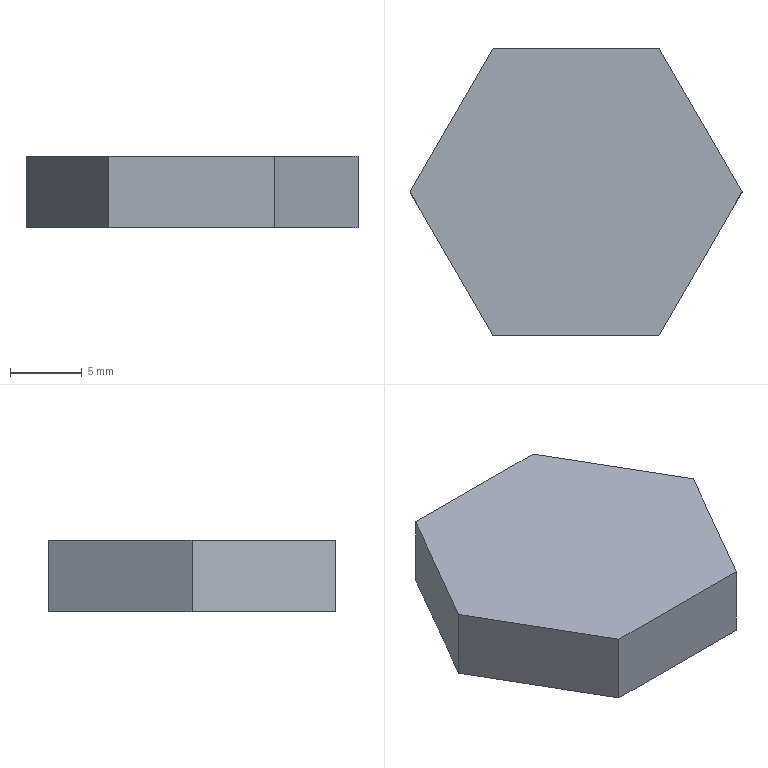Part | NX | features solid 2 | 1 solid | 8 faces | box 23.094 x 20 x 5 mm | volume 1732 mm3 | plane 8
STEP:
#1=CARTESIAN_POINT('',(20.774,205.,0.));
#2=VERTEX_POINT('',#1);
#3=CARTESIAN_POINT('',(9.226,205.,0.));
#4=VERTEX_POINT('',#3);
#5=CARTESIAN_POINT('',(-2.321,205.,0.));
#6=DIRECTION('',(-1.,0.,0.));
#7=VECTOR('',#6,1000.);
#8=LINE('',#5,#7);
#9=EDGE_CURVE('',#2,#4,#8,.T.);
#10=ORIENTED_EDGE('',*,*,#9,.F.);
#11=CARTESIAN_POINT('',(20.774,205.,-5.));
#12=VERTEX_POINT('',#11);
#13=CARTESIAN_POINT('',(20.774,205.,-5.));
#14=DIRECTION('',(0.,0.,1.));
#15=VECTOR('',#14,1000.);
#16=LINE('',#13,#15);
#17=EDGE_CURVE('',#12,#2,#16,.T.);
#18=ORIENTED_EDGE('',*,*,#17,.F.);
#19=CARTESIAN_POINT('',(9.226,205.,-5.));
#20=VERTEX_POINT('',#19);
#21=CARTESIAN_POINT('',(20.774,205.,-5.));
#22=DIRECTION('',(-1.,0.,0.));
#23=VECTOR('',#22,1000.);
#24=LINE('',#21,#23);
#25=EDGE_CURVE('',#12,#20,#24,.T.);
#26=ORIENTED_EDGE('',*,*,#25,.T.);
#27=CARTESIAN_POINT('',(9.226,205.,-5.));
#28=DIRECTION('',(0.,0.,1.));
#29=VECTOR('',#28,1000.);
#30=LINE('',#27,#29);
#31=EDGE_CURVE('',#20,#4,#30,.T.);
#32=ORIENTED_EDGE('',*,*,#31,.T.);
#33=EDGE_LOOP('',(#10,#18,#26,#32));
#34=FACE_BOUND('',#33,.T.);
#35=CARTESIAN_POINT('',(20.774,205.,-5.));
#36=DIRECTION('',(0.,1.,0.));
#37=DIRECTION('',(0.,0.,1.));
#38=AXIS2_PLACEMENT_3D('',#35,#36,#37);
#39=PLANE('',#38);
#40=ADVANCED_FACE('',(#34),#39,.T.);
#41=CARTESIAN_POINT('',(3.453,195.,0.));
#42=VERTEX_POINT('',#41);
#43=CARTESIAN_POINT('',(6.34,200.,0.));
#44=DIRECTION('',(-0.5,-0.866,0.));
#45=VECTOR('',#44,1000.);
#46=LINE('',#43,#45);
#47=EDGE_CURVE('',#4,#42,#46,.T.);
#48=ORIENTED_EDGE('',*,*,#47,.F.);
#49=ORIENTED_EDGE('',*,*,#31,.F.);
#50=CARTESIAN_POINT('',(3.453,195.,-5.));
#51=VERTEX_POINT('',#50);
#52=CARTESIAN_POINT('',(9.226,205.,-5.));
#53=DIRECTION('',(-0.5,-0.866,0.));
#54=VECTOR('',#53,1000.);
#55=LINE('',#52,#54);
#56=EDGE_CURVE('',#20,#51,#55,.T.);
#57=ORIENTED_EDGE('',*,*,#56,.T.);
#58=CARTESIAN_POINT('',(3.453,195.,-5.));
#59=DIRECTION('',(0.,0.,1.));
#60=VECTOR('',#59,1000.);
#61=LINE('',#58,#60);
#62=EDGE_CURVE('',#51,#42,#61,.T.);
#63=ORIENTED_EDGE('',*,*,#62,.T.);
#64=EDGE_LOOP('',(#48,#49,#57,#63));
#65=FACE_BOUND('',#64,.T.);
#66=CARTESIAN_POINT('',(9.226,205.,-5.));
#67=DIRECTION('',(-0.866,0.5,0.));
#68=DIRECTION('',(-0.5,-0.866,0.));
#69=AXIS2_PLACEMENT_3D('',#66,#67,#68);
#70=PLANE('',#69);
#71=ADVANCED_FACE('',(#65),#70,.T.);
#72=CARTESIAN_POINT('',(9.226,185.,0.));
#73=VERTEX_POINT('',#72);
#74=CARTESIAN_POINT('',(-2.321,205.,0.));
#75=DIRECTION('',(0.5,-0.866,0.));
#76=VECTOR('',#75,1000.);
#77=LINE('',#74,#76);
#78=EDGE_CURVE('',#42,#73,#77,.T.);
#79=ORIENTED_EDGE('',*,*,#78,.F.);
#80=ORIENTED_EDGE('',*,*,#62,.F.);
#81=CARTESIAN_POINT('',(9.226,185.,-5.));
#82=VERTEX_POINT('',#81);
#83=CARTESIAN_POINT('',(3.453,195.,-5.));
#84=DIRECTION('',(0.5,-0.866,0.));
#85=VECTOR('',#84,1000.);
#86=LINE('',#83,#85);
#87=EDGE_CURVE('',#51,#82,#86,.T.);
#88=ORIENTED_EDGE('',*,*,#87,.T.);
#89=CARTESIAN_POINT('',(9.226,185.,-5.));
#90=DIRECTION('',(0.,0.,1.));
#91=VECTOR('',#90,1000.);
#92=LINE('',#89,#91);
#93=EDGE_CURVE('',#82,#73,#92,.T.);
#94=ORIENTED_EDGE('',*,*,#93,.T.);
#95=EDGE_LOOP('',(#79,#80,#88,#94));
#96=FACE_BOUND('',#95,.T.);
#97=CARTESIAN_POINT('',(3.453,195.,-5.));
#98=DIRECTION('',(-0.866,-0.5,0.));
#99=DIRECTION('',(0.5,-0.866,0.));
#100=AXIS2_PLACEMENT_3D('',#97,#98,#99);
#101=PLANE('',#100);
#102=ADVANCED_FACE('',(#96),#101,.T.);
#103=CARTESIAN_POINT('',(20.774,185.,0.));
#104=VERTEX_POINT('',#103);
#105=CARTESIAN_POINT('',(-2.321,185.,0.));
#106=DIRECTION('',(1.,0.,0.));
#107=VECTOR('',#106,1000.);
#108=LINE('',#105,#107);
#109=EDGE_CURVE('',#73,#104,#108,.T.);
#110=ORIENTED_EDGE('',*,*,#109,.F.);
#111=ORIENTED_EDGE('',*,*,#93,.F.);
#112=CARTESIAN_POINT('',(20.774,185.,-5.));
#113=VERTEX_POINT('',#112);
#114=CARTESIAN_POINT('',(9.226,185.,-5.));
#115=DIRECTION('',(1.,0.,0.));
#116=VECTOR('',#115,1000.);
#117=LINE('',#114,#116);
#118=EDGE_CURVE('',#82,#113,#117,.T.);
#119=ORIENTED_EDGE('',*,*,#118,.T.);
#120=CARTESIAN_POINT('',(20.774,185.,-5.));
#121=DIRECTION('',(0.,0.,1.));
#122=VECTOR('',#121,1000.);
#123=LINE('',#120,#122);
#124=EDGE_CURVE('',#113,#104,#123,.T.);
#125=ORIENTED_EDGE('',*,*,#124,.T.);
#126=EDGE_LOOP('',(#110,#111,#119,#125));
#127=FACE_BOUND('',#126,.T.);
#128=CARTESIAN_POINT('',(9.226,185.,-5.));
#129=DIRECTION('',(0.,-1.,0.));
#130=DIRECTION('',(1.,0.,0.));
#131=AXIS2_PLACEMENT_3D('',#128,#129,#130);
#132=PLANE('',#131);
#133=ADVANCED_FACE('',(#127),#132,.T.);
#134=CARTESIAN_POINT('',(26.547,195.,0.));
#135=VERTEX_POINT('',#134);
#136=CARTESIAN_POINT('',(23.66,190.,0.));
#137=DIRECTION('',(0.5,0.866,0.));
#138=VECTOR('',#137,1000.);
#139=LINE('',#136,#138);
#140=EDGE_CURVE('',#104,#135,#139,.T.);
#141=ORIENTED_EDGE('',*,*,#140,.F.);
#142=ORIENTED_EDGE('',*,*,#124,.F.);
#143=CARTESIAN_POINT('',(26.547,195.,-5.));
#144=VERTEX_POINT('',#143);
#145=CARTESIAN_POINT('',(20.774,185.,-5.));
#146=DIRECTION('',(0.5,0.866,0.));
#147=VECTOR('',#146,1000.);
#148=LINE('',#145,#147);
#149=EDGE_CURVE('',#113,#144,#148,.T.);
#150=ORIENTED_EDGE('',*,*,#149,.T.);
#151=CARTESIAN_POINT('',(26.547,195.,-5.));
#152=DIRECTION('',(0.,0.,1.));
#153=VECTOR('',#152,1000.);
#154=LINE('',#151,#153);
#155=EDGE_CURVE('',#144,#135,#154,.T.);
#156=ORIENTED_EDGE('',*,*,#155,.T.);
#157=EDGE_LOOP('',(#141,#142,#150,#156));
#158=FACE_BOUND('',#157,.T.);
#159=CARTESIAN_POINT('',(20.774,185.,-5.));
#160=DIRECTION('',(0.866,-0.5,0.));
#161=DIRECTION('',(0.5,0.866,0.));
#162=AXIS2_PLACEMENT_3D('',#159,#160,#161);
#163=PLANE('',#162);
#164=ADVANCED_FACE('',(#158),#163,.T.);
#165=CARTESIAN_POINT('',(15.,215.,0.));
#166=DIRECTION('',(-0.5,0.866,0.));
#167=VECTOR('',#166,1000.);
#168=LINE('',#165,#167);
#169=EDGE_CURVE('',#135,#2,#168,.T.);
#170=ORIENTED_EDGE('',*,*,#169,.F.);
#171=ORIENTED_EDGE('',*,*,#155,.F.);
#172=CARTESIAN_POINT('',(26.547,195.,-5.));
#173=DIRECTION('',(-0.5,0.866,0.));
#174=VECTOR('',#173,1000.);
#175=LINE('',#172,#174);
#176=EDGE_CURVE('',#144,#12,#175,.T.);
#177=ORIENTED_EDGE('',*,*,#176,.T.);
#178=ORIENTED_EDGE('',*,*,#17,.T.);
#179=EDGE_LOOP('',(#170,#171,#177,#178));
#180=FACE_BOUND('',#179,.T.);
#181=CARTESIAN_POINT('',(26.547,195.,-5.));
#182=DIRECTION('',(0.866,0.5,0.));
#183=DIRECTION('',(-0.5,0.866,0.));
#184=AXIS2_PLACEMENT_3D('',#181,#182,#183);
#185=PLANE('',#184);
#186=ADVANCED_FACE('',(#180),#185,.T.);
#187=ORIENTED_EDGE('',*,*,#25,.F.);
#188=ORIENTED_EDGE('',*,*,#176,.F.);
#189=ORIENTED_EDGE('',*,*,#149,.F.);
#190=ORIENTED_EDGE('',*,*,#118,.F.);
#191=ORIENTED_EDGE('',*,*,#87,.F.);
#192=ORIENTED_EDGE('',*,*,#56,.F.);
#193=EDGE_LOOP('',(#187,#188,#189,#190,#191,#192));
#194=FACE_BOUND('',#193,.T.);
#195=CARTESIAN_POINT('',(-2.321,205.,-5.));
#196=DIRECTION('',(0.,0.,1.));
#197=DIRECTION('',(1.,0.,0.));
#198=AXIS2_PLACEMENT_3D('',#195,#196,#197);
#199=PLANE('',#198);
#200=ADVANCED_FACE('',(#194),#199,.F.);
#201=ORIENTED_EDGE('',*,*,#9,.T.);
#202=ORIENTED_EDGE('',*,*,#47,.T.);
#203=ORIENTED_EDGE('',*,*,#78,.T.);
#204=ORIENTED_EDGE('',*,*,#109,.T.);
#205=ORIENTED_EDGE('',*,*,#140,.T.);
#206=ORIENTED_EDGE('',*,*,#169,.T.);
#207=EDGE_LOOP('',(#201,#202,#203,#204,#205,#206));
#208=FACE_BOUND('',#207,.T.);
#209=CARTESIAN_POINT('',(-2.321,205.,0.));
#210=DIRECTION('',(0.,0.,1.));
#211=DIRECTION('',(1.,0.,0.));
#212=AXIS2_PLACEMENT_3D('',#209,#210,#211);
#213=PLANE('',#212);
#214=ADVANCED_FACE('',(#208),#213,.T.);
#215=CLOSED_SHELL('',(#40,#71,#102,#133,#164,#186,#200,#214));
#216=MANIFOLD_SOLID_BREP('',#215);
#217=(LENGTH_UNIT()NAMED_UNIT(*)SI_UNIT(.MILLI.,.METRE.));
#218=UNCERTAINTY_MEASURE_WITH_UNIT(LENGTH_MEASURE(0.00001),#217,'','');
#219=(NAMED_UNIT(*)PLANE_ANGLE_UNIT()SI_UNIT($,.RADIAN.));
#220=(NAMED_UNIT(*)SI_UNIT($,.STERADIAN.)SOLID_ANGLE_UNIT());
#221=(GEOMETRIC_REPRESENTATION_CONTEXT(3)GLOBAL_UNCERTAINTY_ASSIGNED_CONTEXT((#218))GLOBAL_UNIT_ASSIGNED_CONTEXT((#217,#219,#220))REPRESENTATION_CONTEXT('',''));
#222=ADVANCED_BREP_SHAPE_REPRESENTATION('',(#216),#221);